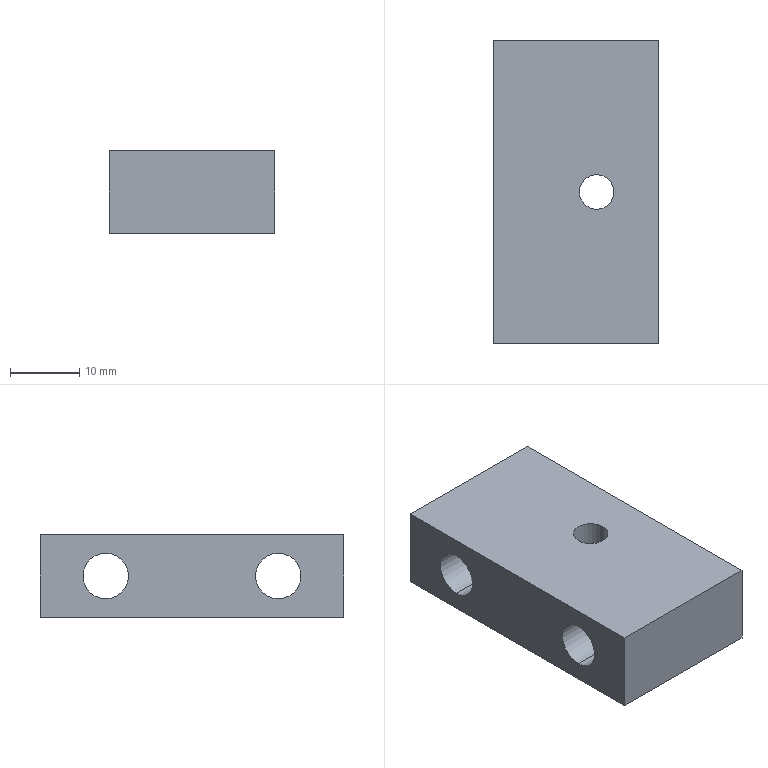Part | STEP file | 1 solid | 18 faces | box 24 x 44 x 12 mm | volume 10016 mm3 | cylinder 10 | plane 8 | commonest cylinder face diameters 6.6 x4 11 x4 5 x2
STEP:
#1=CARTESIAN_POINT('',(0.,0.,0.));
#2=DIRECTION('',(0.,0.,1.));
#3=DIRECTION('',(1.,0.,0.));
#4=AXIS2_PLACEMENT_3D('',#1,#2,#3);
#5=CARTESIAN_POINT('',(17.5,0.,-6.));
#6=VERTEX_POINT('',#5);
#7=CARTESIAN_POINT('',(17.5,0.,6.));
#8=VERTEX_POINT('',#7);
#9=CARTESIAN_POINT('',(17.5,0.,6.));
#10=DIRECTION('',(0.,0.,1.));
#11=VECTOR('',#10,1.);
#12=LINE('',#9,#11);
#13=CARTESIAN_POINT('',(15.,0.,6.));
#14=DIRECTION('',(0.,0.,1.));
#15=DIRECTION('',(1.,0.,0.));
#16=AXIS2_PLACEMENT_3D('',#13,#14,#15);
#17=CYLINDRICAL_SURFACE('',#16,2.5);
#18=CARTESIAN_POINT('',(6.283,0.));
#19=DIRECTION('',(0.,1.));
#20=VECTOR('',#19,1.);
#21=LINE('',#18,#20);
#22=(GEOMETRIC_REPRESENTATION_CONTEXT(2)PARAMETRIC_REPRESENTATION_CONTEXT()REPRESENTATION_CONTEXT('',''));
#23=DEFINITIONAL_REPRESENTATION('',(#21),#22);
#24=PCURVE('',#17,#23);
#25=CARTESIAN_POINT('',(15.,0.,6.));
#26=DIRECTION('',(0.,0.,1.));
#27=DIRECTION('',(1.,0.,0.));
#28=AXIS2_PLACEMENT_3D('',#25,#26,#27);
#29=CYLINDRICAL_SURFACE('',#28,2.5);
#30=CARTESIAN_POINT('',(0.,0.));
#31=DIRECTION('',(0.,1.));
#32=VECTOR('',#31,1.);
#33=LINE('',#30,#32);
#34=(GEOMETRIC_REPRESENTATION_CONTEXT(2)PARAMETRIC_REPRESENTATION_CONTEXT()REPRESENTATION_CONTEXT('',''));
#35=DEFINITIONAL_REPRESENTATION('',(#33),#34);
#36=PCURVE('',#29,#35);
#37=SURFACE_CURVE('',#12,(#24,#36),.PCURVE_S1.);
#38=EDGE_CURVE('',#6,#8,#37,.T.);
#39=ORIENTED_EDGE('',*,*,#38,.T.);
#40=CARTESIAN_POINT('',(12.5,0.,6.));
#41=VERTEX_POINT('',#40);
#42=CARTESIAN_POINT('',(15.,0.,6.));
#43=DIRECTION('',(0.,0.,1.));
#44=DIRECTION('',(1.,0.,0.));
#45=AXIS2_PLACEMENT_3D('',#42,#43,#44);
#46=CIRCLE('',#45,2.5);
#47=CARTESIAN_POINT('',(0.,0.));
#48=DIRECTION('',(1.,0.));
#49=VECTOR('',#48,1.);
#50=LINE('',#47,#49);
#51=(GEOMETRIC_REPRESENTATION_CONTEXT(2)PARAMETRIC_REPRESENTATION_CONTEXT()REPRESENTATION_CONTEXT('',''));
#52=DEFINITIONAL_REPRESENTATION('',(#50),#51);
#53=PCURVE('',#17,#52);
#54=CARTESIAN_POINT('',(24.,-22.,6.));
#55=DIRECTION('',(0.,0.,-1.));
#56=DIRECTION('',(-1.,0.,0.));
#57=AXIS2_PLACEMENT_3D('',#54,#55,#56);
#58=PLANE('',#57);
#59=CARTESIAN_POINT('',(6.5,22.));
#60=CARTESIAN_POINT('',(6.5,26.33));
#61=CARTESIAN_POINT('',(10.25,24.165));
#62=CARTESIAN_POINT('',(14.,22.));
#63=CARTESIAN_POINT('',(10.25,19.835));
#64=CARTESIAN_POINT('',(6.5,17.67));
#65=CARTESIAN_POINT('',(6.5,22.));
#66=(BOUNDED_CURVE()B_SPLINE_CURVE(2,(#59,#60,#61,#62,#63,#64,#65),.UNSPECIFIED.,.T.,.F.)B_SPLINE_CURVE_WITH_KNOTS((1,2,2,2,2,1),(-2.094,0.,2.094,4.189,6.283,8.378),.UNSPECIFIED.)CURVE()GEOMETRIC_REPRESENTATION_ITEM()RATIONAL_B_SPLINE_CURVE((1.,0.5,1.,0.5,1.,0.5,1.))REPRESENTATION_ITEM(''));
#67=(GEOMETRIC_REPRESENTATION_CONTEXT(2)PARAMETRIC_REPRESENTATION_CONTEXT()REPRESENTATION_CONTEXT('',''));
#68=DEFINITIONAL_REPRESENTATION('',(#66),#67);
#69=PCURVE('',#58,#68);
#70=SURFACE_CURVE('',#46,(#53,#69),.PCURVE_S1.);
#71=EDGE_CURVE('',#41,#8,#70,.T.);
#72=ORIENTED_EDGE('',*,*,#71,.F.);
#73=CARTESIAN_POINT('',(12.5,0.,-6.));
#74=VERTEX_POINT('',#73);
#75=CARTESIAN_POINT('',(12.5,0.,6.));
#76=DIRECTION('',(0.,0.,1.));
#77=VECTOR('',#76,1.);
#78=LINE('',#75,#77);
#79=CARTESIAN_POINT('',(3.142,0.));
#80=DIRECTION('',(0.,1.));
#81=VECTOR('',#80,1.);
#82=LINE('',#79,#81);
#83=(GEOMETRIC_REPRESENTATION_CONTEXT(2)PARAMETRIC_REPRESENTATION_CONTEXT()REPRESENTATION_CONTEXT('',''));
#84=DEFINITIONAL_REPRESENTATION('',(#82),#83);
#85=PCURVE('',#17,#84);
#86=CARTESIAN_POINT('',(3.142,0.));
#87=DIRECTION('',(0.,1.));
#88=VECTOR('',#87,1.);
#89=LINE('',#86,#88);
#90=(GEOMETRIC_REPRESENTATION_CONTEXT(2)PARAMETRIC_REPRESENTATION_CONTEXT()REPRESENTATION_CONTEXT('',''));
#91=DEFINITIONAL_REPRESENTATION('',(#89),#90);
#92=PCURVE('',#29,#91);
#93=SURFACE_CURVE('',#78,(#85,#92),.PCURVE_S1.);
#94=EDGE_CURVE('',#74,#41,#93,.T.);
#95=ORIENTED_EDGE('',*,*,#94,.F.);
#96=CARTESIAN_POINT('',(15.,0.,-6.));
#97=DIRECTION('',(0.,0.,1.));
#98=DIRECTION('',(1.,0.,0.));
#99=AXIS2_PLACEMENT_3D('',#96,#97,#98);
#100=CIRCLE('',#99,2.5);
#101=CARTESIAN_POINT('',(0.,-12.));
#102=DIRECTION('',(1.,0.));
#103=VECTOR('',#102,1.);
#104=LINE('',#101,#103);
#105=(GEOMETRIC_REPRESENTATION_CONTEXT(2)PARAMETRIC_REPRESENTATION_CONTEXT()REPRESENTATION_CONTEXT('',''));
#106=DEFINITIONAL_REPRESENTATION('',(#104),#105);
#107=PCURVE('',#17,#106);
#108=CARTESIAN_POINT('',(24.,-22.,-6.));
#109=DIRECTION('',(0.,0.,1.));
#110=DIRECTION('',(1.,0.,0.));
#111=AXIS2_PLACEMENT_3D('',#108,#109,#110);
#112=PLANE('',#111);
#113=CARTESIAN_POINT('',(-9.,22.));
#114=DIRECTION('',(1.,0.));
#115=AXIS2_PLACEMENT_2D('',#113,#114);
#116=CIRCLE('',#115,2.5);
#117=(GEOMETRIC_REPRESENTATION_CONTEXT(2)PARAMETRIC_REPRESENTATION_CONTEXT()REPRESENTATION_CONTEXT('',''));
#118=DEFINITIONAL_REPRESENTATION('',(#116),#117);
#119=PCURVE('',#112,#118);
#120=SURFACE_CURVE('',#100,(#107,#119),.PCURVE_S1.);
#121=EDGE_CURVE('',#74,#6,#120,.T.);
#122=ORIENTED_EDGE('',*,*,#121,.T.);
#123=EDGE_LOOP('',(#39,#72,#95,#122));
#124=FACE_BOUND('',#123,.F.);
#125=ADVANCED_FACE('',(#124),#17,.F.);
#126=CARTESIAN_POINT('',(17.6,12.5,-5.5));
#127=VERTEX_POINT('',#126);
#128=CARTESIAN_POINT('',(24.,12.5,-5.5));
#129=VERTEX_POINT('',#128);
#130=CARTESIAN_POINT('',(24.,12.5,-5.5));
#131=DIRECTION('',(1.,0.,0.));
#132=VECTOR('',#131,1.);
#133=LINE('',#130,#132);
#134=CARTESIAN_POINT('',(24.,12.5,0.));
#135=DIRECTION('',(1.,0.,0.));
#136=DIRECTION('',(0.,0.,-1.));
#137=AXIS2_PLACEMENT_3D('',#134,#135,#136);
#138=CYLINDRICAL_SURFACE('',#137,5.5);
#139=CARTESIAN_POINT('',(6.283,0.));
#140=DIRECTION('',(0.,1.));
#141=VECTOR('',#140,1.);
#142=LINE('',#139,#141);
#143=(GEOMETRIC_REPRESENTATION_CONTEXT(2)PARAMETRIC_REPRESENTATION_CONTEXT()REPRESENTATION_CONTEXT('',''));
#144=DEFINITIONAL_REPRESENTATION('',(#142),#143);
#145=PCURVE('',#138,#144);
#146=CARTESIAN_POINT('',(24.,12.5,0.));
#147=DIRECTION('',(1.,0.,0.));
#148=DIRECTION('',(0.,0.,-1.));
#149=AXIS2_PLACEMENT_3D('',#146,#147,#148);
#150=CYLINDRICAL_SURFACE('',#149,5.5);
#151=CARTESIAN_POINT('',(0.,0.));
#152=DIRECTION('',(0.,1.));
#153=VECTOR('',#152,1.);
#154=LINE('',#151,#153);
#155=(GEOMETRIC_REPRESENTATION_CONTEXT(2)PARAMETRIC_REPRESENTATION_CONTEXT()REPRESENTATION_CONTEXT('',''));
#156=DEFINITIONAL_REPRESENTATION('',(#154),#155);
#157=PCURVE('',#150,#156);
#158=SURFACE_CURVE('',#133,(#145,#157),.PCURVE_S1.);
#159=EDGE_CURVE('',#127,#129,#158,.T.);
#160=ORIENTED_EDGE('',*,*,#159,.T.);
#161=CARTESIAN_POINT('',(24.,12.5,5.5));
#162=VERTEX_POINT('',#161);
#163=CARTESIAN_POINT('',(24.,12.5,0.));
#164=DIRECTION('',(1.,0.,0.));
#165=DIRECTION('',(0.,0.,-1.));
#166=AXIS2_PLACEMENT_3D('',#163,#164,#165);
#167=CIRCLE('',#166,5.5);
#168=CARTESIAN_POINT('',(0.,0.));
#169=DIRECTION('',(1.,0.));
#170=VECTOR('',#169,1.);
#171=LINE('',#168,#170);
#172=(GEOMETRIC_REPRESENTATION_CONTEXT(2)PARAMETRIC_REPRESENTATION_CONTEXT()REPRESENTATION_CONTEXT('',''));
#173=DEFINITIONAL_REPRESENTATION('',(#171),#172);
#174=PCURVE('',#138,#173);
#175=CARTESIAN_POINT('',(24.,0.,0.));
#176=DIRECTION('',(1.,0.,0.));
#177=DIRECTION('',(0.,0.,-1.));
#178=AXIS2_PLACEMENT_3D('',#175,#176,#177);
#179=PLANE('',#178);
#180=CARTESIAN_POINT('',(0.,12.5));
#181=DIRECTION('',(1.,0.));
#182=AXIS2_PLACEMENT_2D('',#180,#181);
#183=CIRCLE('',#182,5.5);
#184=(GEOMETRIC_REPRESENTATION_CONTEXT(2)PARAMETRIC_REPRESENTATION_CONTEXT()REPRESENTATION_CONTEXT('',''));
#185=DEFINITIONAL_REPRESENTATION('',(#183),#184);
#186=PCURVE('',#179,#185);
#187=SURFACE_CURVE('',#167,(#174,#186),.PCURVE_S1.);
#188=EDGE_CURVE('',#162,#129,#187,.T.);
#189=ORIENTED_EDGE('',*,*,#188,.F.);
#190=CARTESIAN_POINT('',(17.6,12.5,5.5));
#191=VERTEX_POINT('',#190);
#192=CARTESIAN_POINT('',(24.,12.5,5.5));
#193=DIRECTION('',(1.,0.,0.));
#194=VECTOR('',#193,1.);
#195=LINE('',#192,#194);
#196=CARTESIAN_POINT('',(3.142,0.));
#197=DIRECTION('',(0.,1.));
#198=VECTOR('',#197,1.);
#199=LINE('',#196,#198);
#200=(GEOMETRIC_REPRESENTATION_CONTEXT(2)PARAMETRIC_REPRESENTATION_CONTEXT()REPRESENTATION_CONTEXT('',''));
#201=DEFINITIONAL_REPRESENTATION('',(#199),#200);
#202=PCURVE('',#138,#201);
#203=CARTESIAN_POINT('',(3.142,0.));
#204=DIRECTION('',(0.,1.));
#205=VECTOR('',#204,1.);
#206=LINE('',#203,#205);
#207=(GEOMETRIC_REPRESENTATION_CONTEXT(2)PARAMETRIC_REPRESENTATION_CONTEXT()REPRESENTATION_CONTEXT('',''));
#208=DEFINITIONAL_REPRESENTATION('',(#206),#207);
#209=PCURVE('',#150,#208);
#210=SURFACE_CURVE('',#195,(#202,#209),.PCURVE_S1.);
#211=EDGE_CURVE('',#191,#162,#210,.T.);
#212=ORIENTED_EDGE('',*,*,#211,.F.);
#213=CARTESIAN_POINT('',(17.6,12.5,0.));
#214=DIRECTION('',(1.,0.,0.));
#215=DIRECTION('',(0.,0.,-1.));
#216=AXIS2_PLACEMENT_3D('',#213,#214,#215);
#217=CIRCLE('',#216,5.5);
#218=CARTESIAN_POINT('',(0.,-6.4));
#219=DIRECTION('',(1.,0.));
#220=VECTOR('',#219,1.);
#221=LINE('',#218,#220);
#222=(GEOMETRIC_REPRESENTATION_CONTEXT(2)PARAMETRIC_REPRESENTATION_CONTEXT()REPRESENTATION_CONTEXT('',''));
#223=DEFINITIONAL_REPRESENTATION('',(#221),#222);
#224=PCURVE('',#138,#223);
#225=CARTESIAN_POINT('',(17.6,15.8,0.));
#226=DIRECTION('',(-1.,0.,0.));
#227=DIRECTION('',(0.,0.,1.));
#228=AXIS2_PLACEMENT_3D('',#225,#226,#227);
#229=PLANE('',#228);
#230=CARTESIAN_POINT('',(-5.5,-3.3));
#231=CARTESIAN_POINT('',(-5.5,6.226));
#232=CARTESIAN_POINT('',(2.75,1.463));
#233=CARTESIAN_POINT('',(11.,-3.3));
#234=CARTESIAN_POINT('',(2.75,-8.063));
#235=CARTESIAN_POINT('',(-5.5,-12.826));
#236=CARTESIAN_POINT('',(-5.5,-3.3));
#237=(BOUNDED_CURVE()B_SPLINE_CURVE(2,(#230,#231,#232,#233,#234,#235,#236),.UNSPECIFIED.,.T.,.F.)B_SPLINE_CURVE_WITH_KNOTS((1,2,2,2,2,1),(-2.094,0.,2.094,4.189,6.283,8.378),.UNSPECIFIED.)CURVE()GEOMETRIC_REPRESENTATION_ITEM()RATIONAL_B_SPLINE_CURVE((1.,0.5,1.,0.5,1.,0.5,1.))REPRESENTATION_ITEM(''));
#238=(GEOMETRIC_REPRESENTATION_CONTEXT(2)PARAMETRIC_REPRESENTATION_CONTEXT()REPRESENTATION_CONTEXT('',''));
#239=DEFINITIONAL_REPRESENTATION('',(#237),#238);
#240=PCURVE('',#229,#239);
#241=SURFACE_CURVE('',#217,(#224,#240),.PCURVE_S1.);
#242=EDGE_CURVE('',#191,#127,#241,.T.);
#243=ORIENTED_EDGE('',*,*,#242,.T.);
#244=EDGE_LOOP('',(#160,#189,#212,#243));
#245=FACE_BOUND('',#244,.F.);
#246=ADVANCED_FACE('',(#245),#138,.F.);
#247=CARTESIAN_POINT('',(0.,12.5,-3.3));
#248=VERTEX_POINT('',#247);
#249=CARTESIAN_POINT('',(17.6,12.5,-3.3));
#250=VERTEX_POINT('',#249);
#251=CARTESIAN_POINT('',(24.,12.5,-3.3));
#252=DIRECTION('',(1.,0.,0.));
#253=VECTOR('',#252,1.);
#254=LINE('',#251,#253);
#255=CARTESIAN_POINT('',(24.,12.5,0.));
#256=DIRECTION('',(1.,0.,0.));
#257=DIRECTION('',(0.,0.,-1.));
#258=AXIS2_PLACEMENT_3D('',#255,#256,#257);
#259=CYLINDRICAL_SURFACE('',#258,3.3);
#260=CARTESIAN_POINT('',(6.283,0.));
#261=DIRECTION('',(0.,1.));
#262=VECTOR('',#261,1.);
#263=LINE('',#260,#262);
#264=(GEOMETRIC_REPRESENTATION_CONTEXT(2)PARAMETRIC_REPRESENTATION_CONTEXT()REPRESENTATION_CONTEXT('',''));
#265=DEFINITIONAL_REPRESENTATION('',(#263),#264);
#266=PCURVE('',#259,#265);
#267=CARTESIAN_POINT('',(24.,12.5,0.));
#268=DIRECTION('',(1.,0.,0.));
#269=DIRECTION('',(0.,0.,-1.));
#270=AXIS2_PLACEMENT_3D('',#267,#268,#269);
#271=CYLINDRICAL_SURFACE('',#270,3.3);
#272=CARTESIAN_POINT('',(0.,0.));
#273=DIRECTION('',(0.,1.));
#274=VECTOR('',#273,1.);
#275=LINE('',#272,#274);
#276=(GEOMETRIC_REPRESENTATION_CONTEXT(2)PARAMETRIC_REPRESENTATION_CONTEXT()REPRESENTATION_CONTEXT('',''));
#277=DEFINITIONAL_REPRESENTATION('',(#275),#276);
#278=PCURVE('',#271,#277);
#279=SURFACE_CURVE('',#254,(#266,#278),.PCURVE_S1.);
#280=EDGE_CURVE('',#248,#250,#279,.T.);
#281=ORIENTED_EDGE('',*,*,#280,.T.);
#282=CARTESIAN_POINT('',(17.6,12.5,3.3));
#283=VERTEX_POINT('',#282);
#284=CARTESIAN_POINT('',(17.6,12.5,0.));
#285=DIRECTION('',(1.,0.,0.));
#286=DIRECTION('',(0.,0.,-1.));
#287=AXIS2_PLACEMENT_3D('',#284,#285,#286);
#288=CIRCLE('',#287,3.3);
#289=CARTESIAN_POINT('',(0.,-6.4));
#290=DIRECTION('',(1.,0.));
#291=VECTOR('',#290,1.);
#292=LINE('',#289,#291);
#293=(GEOMETRIC_REPRESENTATION_CONTEXT(2)PARAMETRIC_REPRESENTATION_CONTEXT()REPRESENTATION_CONTEXT('',''));
#294=DEFINITIONAL_REPRESENTATION('',(#292),#293);
#295=PCURVE('',#259,#294);
#296=CARTESIAN_POINT('',(-3.3,-3.3));
#297=CARTESIAN_POINT('',(-3.3,2.416));
#298=CARTESIAN_POINT('',(1.65,-0.4421));
#299=CARTESIAN_POINT('',(6.6,-3.3));
#300=CARTESIAN_POINT('',(1.65,-6.158));
#301=CARTESIAN_POINT('',(-3.3,-9.016));
#302=CARTESIAN_POINT('',(-3.3,-3.3));
#303=(BOUNDED_CURVE()B_SPLINE_CURVE(2,(#296,#297,#298,#299,#300,#301,#302),.UNSPECIFIED.,.T.,.F.)B_SPLINE_CURVE_WITH_KNOTS((1,2,2,2,2,1),(-2.094,0.,2.094,4.189,6.283,8.378),.UNSPECIFIED.)CURVE()GEOMETRIC_REPRESENTATION_ITEM()RATIONAL_B_SPLINE_CURVE((1.,0.5,1.,0.5,1.,0.5,1.))REPRESENTATION_ITEM(''));
#304=(GEOMETRIC_REPRESENTATION_CONTEXT(2)PARAMETRIC_REPRESENTATION_CONTEXT()REPRESENTATION_CONTEXT('',''));
#305=DEFINITIONAL_REPRESENTATION('',(#303),#304);
#306=PCURVE('',#229,#305);
#307=SURFACE_CURVE('',#288,(#295,#306),.PCURVE_S1.);
#308=EDGE_CURVE('',#283,#250,#307,.T.);
#309=ORIENTED_EDGE('',*,*,#308,.F.);
#310=CARTESIAN_POINT('',(0.,12.5,3.3));
#311=VERTEX_POINT('',#310);
#312=CARTESIAN_POINT('',(24.,12.5,3.3));
#313=DIRECTION('',(1.,0.,0.));
#314=VECTOR('',#313,1.);
#315=LINE('',#312,#314);
#316=CARTESIAN_POINT('',(3.142,0.));
#317=DIRECTION('',(0.,1.));
#318=VECTOR('',#317,1.);
#319=LINE('',#316,#318);
#320=(GEOMETRIC_REPRESENTATION_CONTEXT(2)PARAMETRIC_REPRESENTATION_CONTEXT()REPRESENTATION_CONTEXT('',''));
#321=DEFINITIONAL_REPRESENTATION('',(#319),#320);
#322=PCURVE('',#259,#321);
#323=CARTESIAN_POINT('',(3.142,0.));
#324=DIRECTION('',(0.,1.));
#325=VECTOR('',#324,1.);
#326=LINE('',#323,#325);
#327=(GEOMETRIC_REPRESENTATION_CONTEXT(2)PARAMETRIC_REPRESENTATION_CONTEXT()REPRESENTATION_CONTEXT('',''));
#328=DEFINITIONAL_REPRESENTATION('',(#326),#327);
#329=PCURVE('',#271,#328);
#330=SURFACE_CURVE('',#315,(#322,#329),.PCURVE_S1.);
#331=EDGE_CURVE('',#311,#283,#330,.T.);
#332=ORIENTED_EDGE('',*,*,#331,.F.);
#333=CARTESIAN_POINT('',(0.,12.5,0.));
#334=DIRECTION('',(1.,0.,0.));
#335=DIRECTION('',(0.,0.,-1.));
#336=AXIS2_PLACEMENT_3D('',#333,#334,#335);
#337=CIRCLE('',#336,3.3);
#338=CARTESIAN_POINT('',(0.,-24.));
#339=DIRECTION('',(1.,0.));
#340=VECTOR('',#339,1.);
#341=LINE('',#338,#340);
#342=(GEOMETRIC_REPRESENTATION_CONTEXT(2)PARAMETRIC_REPRESENTATION_CONTEXT()REPRESENTATION_CONTEXT('',''));
#343=DEFINITIONAL_REPRESENTATION('',(#341),#342);
#344=PCURVE('',#259,#343);
#345=CARTESIAN_POINT('',(0.,0.,0.));
#346=DIRECTION('',(1.,0.,0.));
#347=DIRECTION('',(0.,0.,-1.));
#348=AXIS2_PLACEMENT_3D('',#345,#346,#347);
#349=PLANE('',#348);
#350=CARTESIAN_POINT('',(0.,12.5));
#351=DIRECTION('',(1.,0.));
#352=AXIS2_PLACEMENT_2D('',#350,#351);
#353=CIRCLE('',#352,3.3);
#354=(GEOMETRIC_REPRESENTATION_CONTEXT(2)PARAMETRIC_REPRESENTATION_CONTEXT()REPRESENTATION_CONTEXT('',''));
#355=DEFINITIONAL_REPRESENTATION('',(#353),#354);
#356=PCURVE('',#349,#355);
#357=SURFACE_CURVE('',#337,(#344,#356),.PCURVE_S1.);
#358=EDGE_CURVE('',#311,#248,#357,.T.);
#359=ORIENTED_EDGE('',*,*,#358,.T.);
#360=EDGE_LOOP('',(#281,#309,#332,#359));
#361=FACE_BOUND('',#360,.F.);
#362=ADVANCED_FACE('',(#361),#259,.F.);
#363=CARTESIAN_POINT('',(17.6,-12.5,-5.5));
#364=VERTEX_POINT('',#363);
#365=CARTESIAN_POINT('',(24.,-12.5,-5.5));
#366=VERTEX_POINT('',#365);
#367=CARTESIAN_POINT('',(24.,-12.5,-5.5));
#368=DIRECTION('',(1.,0.,0.));
#369=VECTOR('',#368,1.);
#370=LINE('',#367,#369);
#371=CARTESIAN_POINT('',(24.,-12.5,0.));
#372=DIRECTION('',(1.,0.,0.));
#373=DIRECTION('',(0.,0.,-1.));
#374=AXIS2_PLACEMENT_3D('',#371,#372,#373);
#375=CYLINDRICAL_SURFACE('',#374,5.5);
#376=CARTESIAN_POINT('',(6.283,0.));
#377=DIRECTION('',(0.,1.));
#378=VECTOR('',#377,1.);
#379=LINE('',#376,#378);
#380=(GEOMETRIC_REPRESENTATION_CONTEXT(2)PARAMETRIC_REPRESENTATION_CONTEXT()REPRESENTATION_CONTEXT('',''));
#381=DEFINITIONAL_REPRESENTATION('',(#379),#380);
#382=PCURVE('',#375,#381);
#383=CARTESIAN_POINT('',(24.,-12.5,0.));
#384=DIRECTION('',(1.,0.,0.));
#385=DIRECTION('',(0.,0.,-1.));
#386=AXIS2_PLACEMENT_3D('',#383,#384,#385);
#387=CYLINDRICAL_SURFACE('',#386,5.5);
#388=CARTESIAN_POINT('',(0.,0.));
#389=DIRECTION('',(0.,1.));
#390=VECTOR('',#389,1.);
#391=LINE('',#388,#390);
#392=(GEOMETRIC_REPRESENTATION_CONTEXT(2)PARAMETRIC_REPRESENTATION_CONTEXT()REPRESENTATION_CONTEXT('',''));
#393=DEFINITIONAL_REPRESENTATION('',(#391),#392);
#394=PCURVE('',#387,#393);
#395=SURFACE_CURVE('',#370,(#382,#394),.PCURVE_S1.);
#396=EDGE_CURVE('',#364,#366,#395,.T.);
#397=ORIENTED_EDGE('',*,*,#396,.T.);
#398=CARTESIAN_POINT('',(24.,-12.5,5.5));
#399=VERTEX_POINT('',#398);
#400=CARTESIAN_POINT('',(24.,-12.5,0.));
#401=DIRECTION('',(1.,0.,0.));
#402=DIRECTION('',(0.,0.,-1.));
#403=AXIS2_PLACEMENT_3D('',#400,#401,#402);
#404=CIRCLE('',#403,5.5);
#405=CARTESIAN_POINT('',(0.,0.));
#406=DIRECTION('',(1.,0.));
#407=VECTOR('',#406,1.);
#408=LINE('',#405,#407);
#409=(GEOMETRIC_REPRESENTATION_CONTEXT(2)PARAMETRIC_REPRESENTATION_CONTEXT()REPRESENTATION_CONTEXT('',''));
#410=DEFINITIONAL_REPRESENTATION('',(#408),#409);
#411=PCURVE('',#375,#410);
#412=CARTESIAN_POINT('',(0.,-12.5));
#413=DIRECTION('',(1.,0.));
#414=AXIS2_PLACEMENT_2D('',#412,#413);
#415=CIRCLE('',#414,5.5);
#416=(GEOMETRIC_REPRESENTATION_CONTEXT(2)PARAMETRIC_REPRESENTATION_CONTEXT()REPRESENTATION_CONTEXT('',''));
#417=DEFINITIONAL_REPRESENTATION('',(#415),#416);
#418=PCURVE('',#179,#417);
#419=SURFACE_CURVE('',#404,(#411,#418),.PCURVE_S1.);
#420=EDGE_CURVE('',#399,#366,#419,.T.);
#421=ORIENTED_EDGE('',*,*,#420,.F.);
#422=CARTESIAN_POINT('',(17.6,-12.5,5.5));
#423=VERTEX_POINT('',#422);
#424=CARTESIAN_POINT('',(24.,-12.5,5.5));
#425=DIRECTION('',(1.,0.,0.));
#426=VECTOR('',#425,1.);
#427=LINE('',#424,#426);
#428=CARTESIAN_POINT('',(3.142,0.));
#429=DIRECTION('',(0.,1.));
#430=VECTOR('',#429,1.);
#431=LINE('',#428,#430);
#432=(GEOMETRIC_REPRESENTATION_CONTEXT(2)PARAMETRIC_REPRESENTATION_CONTEXT()REPRESENTATION_CONTEXT('',''));
#433=DEFINITIONAL_REPRESENTATION('',(#431),#432);
#434=PCURVE('',#375,#433);
#435=CARTESIAN_POINT('',(3.142,0.));
#436=DIRECTION('',(0.,1.));
#437=VECTOR('',#436,1.);
#438=LINE('',#435,#437);
#439=(GEOMETRIC_REPRESENTATION_CONTEXT(2)PARAMETRIC_REPRESENTATION_CONTEXT()REPRESENTATION_CONTEXT('',''));
#440=DEFINITIONAL_REPRESENTATION('',(#438),#439);
#441=PCURVE('',#387,#440);
#442=SURFACE_CURVE('',#427,(#434,#441),.PCURVE_S1.);
#443=EDGE_CURVE('',#423,#399,#442,.T.);
#444=ORIENTED_EDGE('',*,*,#443,.F.);
#445=CARTESIAN_POINT('',(17.6,-12.5,0.));
#446=DIRECTION('',(1.,0.,0.));
#447=DIRECTION('',(0.,0.,-1.));
#448=AXIS2_PLACEMENT_3D('',#445,#446,#447);
#449=CIRCLE('',#448,5.5);
#450=CARTESIAN_POINT('',(0.,-6.4));
#451=DIRECTION('',(1.,0.));
#452=VECTOR('',#451,1.);
#453=LINE('',#450,#452);
#454=(GEOMETRIC_REPRESENTATION_CONTEXT(2)PARAMETRIC_REPRESENTATION_CONTEXT()REPRESENTATION_CONTEXT('',''));
#455=DEFINITIONAL_REPRESENTATION('',(#453),#454);
#456=PCURVE('',#375,#455);
#457=CARTESIAN_POINT('',(17.6,-9.2,0.));
#458=DIRECTION('',(-1.,0.,0.));
#459=DIRECTION('',(0.,0.,1.));
#460=AXIS2_PLACEMENT_3D('',#457,#458,#459);
#461=PLANE('',#460);
#462=CARTESIAN_POINT('',(-5.5,-3.3));
#463=CARTESIAN_POINT('',(-5.5,6.226));
#464=CARTESIAN_POINT('',(2.75,1.463));
#465=CARTESIAN_POINT('',(11.,-3.3));
#466=CARTESIAN_POINT('',(2.75,-8.063));
#467=CARTESIAN_POINT('',(-5.5,-12.826));
#468=CARTESIAN_POINT('',(-5.5,-3.3));
#469=(BOUNDED_CURVE()B_SPLINE_CURVE(2,(#462,#463,#464,#465,#466,#467,#468),.UNSPECIFIED.,.T.,.F.)B_SPLINE_CURVE_WITH_KNOTS((1,2,2,2,2,1),(-2.094,0.,2.094,4.189,6.283,8.378),.UNSPECIFIED.)CURVE()GEOMETRIC_REPRESENTATION_ITEM()RATIONAL_B_SPLINE_CURVE((1.,0.5,1.,0.5,1.,0.5,1.))REPRESENTATION_ITEM(''));
#470=(GEOMETRIC_REPRESENTATION_CONTEXT(2)PARAMETRIC_REPRESENTATION_CONTEXT()REPRESENTATION_CONTEXT('',''));
#471=DEFINITIONAL_REPRESENTATION('',(#469),#470);
#472=PCURVE('',#461,#471);
#473=SURFACE_CURVE('',#449,(#456,#472),.PCURVE_S1.);
#474=EDGE_CURVE('',#423,#364,#473,.T.);
#475=ORIENTED_EDGE('',*,*,#474,.T.);
#476=EDGE_LOOP('',(#397,#421,#444,#475));
#477=FACE_BOUND('',#476,.F.);
#478=ADVANCED_FACE('',(#477),#375,.F.);
#479=CARTESIAN_POINT('',(0.,-12.5,-3.3));
#480=VERTEX_POINT('',#479);
#481=CARTESIAN_POINT('',(17.6,-12.5,-3.3));
#482=VERTEX_POINT('',#481);
#483=CARTESIAN_POINT('',(24.,-12.5,-3.3));
#484=DIRECTION('',(1.,0.,0.));
#485=VECTOR('',#484,1.);
#486=LINE('',#483,#485);
#487=CARTESIAN_POINT('',(24.,-12.5,0.));
#488=DIRECTION('',(1.,0.,0.));
#489=DIRECTION('',(0.,0.,-1.));
#490=AXIS2_PLACEMENT_3D('',#487,#488,#489);
#491=CYLINDRICAL_SURFACE('',#490,3.3);
#492=CARTESIAN_POINT('',(6.283,0.));
#493=DIRECTION('',(0.,1.));
#494=VECTOR('',#493,1.);
#495=LINE('',#492,#494);
#496=(GEOMETRIC_REPRESENTATION_CONTEXT(2)PARAMETRIC_REPRESENTATION_CONTEXT()REPRESENTATION_CONTEXT('',''));
#497=DEFINITIONAL_REPRESENTATION('',(#495),#496);
#498=PCURVE('',#491,#497);
#499=CARTESIAN_POINT('',(24.,-12.5,0.));
#500=DIRECTION('',(1.,0.,0.));
#501=DIRECTION('',(0.,0.,-1.));
#502=AXIS2_PLACEMENT_3D('',#499,#500,#501);
#503=CYLINDRICAL_SURFACE('',#502,3.3);
#504=CARTESIAN_POINT('',(0.,0.));
#505=DIRECTION('',(0.,1.));
#506=VECTOR('',#505,1.);
#507=LINE('',#504,#506);
#508=(GEOMETRIC_REPRESENTATION_CONTEXT(2)PARAMETRIC_REPRESENTATION_CONTEXT()REPRESENTATION_CONTEXT('',''));
#509=DEFINITIONAL_REPRESENTATION('',(#507),#508);
#510=PCURVE('',#503,#509);
#511=SURFACE_CURVE('',#486,(#498,#510),.PCURVE_S1.);
#512=EDGE_CURVE('',#480,#482,#511,.T.);
#513=ORIENTED_EDGE('',*,*,#512,.T.);
#514=CARTESIAN_POINT('',(17.6,-12.5,3.3));
#515=VERTEX_POINT('',#514);
#516=CARTESIAN_POINT('',(17.6,-12.5,0.));
#517=DIRECTION('',(1.,0.,0.));
#518=DIRECTION('',(0.,0.,-1.));
#519=AXIS2_PLACEMENT_3D('',#516,#517,#518);
#520=CIRCLE('',#519,3.3);
#521=CARTESIAN_POINT('',(0.,-6.4));
#522=DIRECTION('',(1.,0.));
#523=VECTOR('',#522,1.);
#524=LINE('',#521,#523);
#525=(GEOMETRIC_REPRESENTATION_CONTEXT(2)PARAMETRIC_REPRESENTATION_CONTEXT()REPRESENTATION_CONTEXT('',''));
#526=DEFINITIONAL_REPRESENTATION('',(#524),#525);
#527=PCURVE('',#491,#526);
#528=CARTESIAN_POINT('',(-3.3,-3.3));
#529=CARTESIAN_POINT('',(-3.3,2.416));
#530=CARTESIAN_POINT('',(1.65,-0.4421));
#531=CARTESIAN_POINT('',(6.6,-3.3));
#532=CARTESIAN_POINT('',(1.65,-6.158));
#533=CARTESIAN_POINT('',(-3.3,-9.016));
#534=CARTESIAN_POINT('',(-3.3,-3.3));
#535=(BOUNDED_CURVE()B_SPLINE_CURVE(2,(#528,#529,#530,#531,#532,#533,#534),.UNSPECIFIED.,.T.,.F.)B_SPLINE_CURVE_WITH_KNOTS((1,2,2,2,2,1),(-2.094,0.,2.094,4.189,6.283,8.378),.UNSPECIFIED.)CURVE()GEOMETRIC_REPRESENTATION_ITEM()RATIONAL_B_SPLINE_CURVE((1.,0.5,1.,0.5,1.,0.5,1.))REPRESENTATION_ITEM(''));
#536=(GEOMETRIC_REPRESENTATION_CONTEXT(2)PARAMETRIC_REPRESENTATION_CONTEXT()REPRESENTATION_CONTEXT('',''));
#537=DEFINITIONAL_REPRESENTATION('',(#535),#536);
#538=PCURVE('',#461,#537);
#539=SURFACE_CURVE('',#520,(#527,#538),.PCURVE_S1.);
#540=EDGE_CURVE('',#515,#482,#539,.T.);
#541=ORIENTED_EDGE('',*,*,#540,.F.);
#542=CARTESIAN_POINT('',(0.,-12.5,3.3));
#543=VERTEX_POINT('',#542);
#544=CARTESIAN_POINT('',(24.,-12.5,3.3));
#545=DIRECTION('',(1.,0.,0.));
#546=VECTOR('',#545,1.);
#547=LINE('',#544,#546);
#548=CARTESIAN_POINT('',(3.142,0.));
#549=DIRECTION('',(0.,1.));
#550=VECTOR('',#549,1.);
#551=LINE('',#548,#550);
#552=(GEOMETRIC_REPRESENTATION_CONTEXT(2)PARAMETRIC_REPRESENTATION_CONTEXT()REPRESENTATION_CONTEXT('',''));
#553=DEFINITIONAL_REPRESENTATION('',(#551),#552);
#554=PCURVE('',#491,#553);
#555=CARTESIAN_POINT('',(3.142,0.));
#556=DIRECTION('',(0.,1.));
#557=VECTOR('',#556,1.);
#558=LINE('',#555,#557);
#559=(GEOMETRIC_REPRESENTATION_CONTEXT(2)PARAMETRIC_REPRESENTATION_CONTEXT()REPRESENTATION_CONTEXT('',''));
#560=DEFINITIONAL_REPRESENTATION('',(#558),#559);
#561=PCURVE('',#503,#560);
#562=SURFACE_CURVE('',#547,(#554,#561),.PCURVE_S1.);
#563=EDGE_CURVE('',#543,#515,#562,.T.);
#564=ORIENTED_EDGE('',*,*,#563,.F.);
#565=CARTESIAN_POINT('',(0.,-12.5,0.));
#566=DIRECTION('',(1.,0.,0.));
#567=DIRECTION('',(0.,0.,-1.));
#568=AXIS2_PLACEMENT_3D('',#565,#566,#567);
#569=CIRCLE('',#568,3.3);
#570=CARTESIAN_POINT('',(0.,-24.));
#571=DIRECTION('',(1.,0.));
#572=VECTOR('',#571,1.);
#573=LINE('',#570,#572);
#574=(GEOMETRIC_REPRESENTATION_CONTEXT(2)PARAMETRIC_REPRESENTATION_CONTEXT()REPRESENTATION_CONTEXT('',''));
#575=DEFINITIONAL_REPRESENTATION('',(#573),#574);
#576=PCURVE('',#491,#575);
#577=CARTESIAN_POINT('',(0.,-12.5));
#578=DIRECTION('',(1.,0.));
#579=AXIS2_PLACEMENT_2D('',#577,#578);
#580=CIRCLE('',#579,3.3);
#581=(GEOMETRIC_REPRESENTATION_CONTEXT(2)PARAMETRIC_REPRESENTATION_CONTEXT()REPRESENTATION_CONTEXT('',''));
#582=DEFINITIONAL_REPRESENTATION('',(#580),#581);
#583=PCURVE('',#349,#582);
#584=SURFACE_CURVE('',#569,(#576,#583),.PCURVE_S1.);
#585=EDGE_CURVE('',#543,#480,#584,.T.);
#586=ORIENTED_EDGE('',*,*,#585,.T.);
#587=EDGE_LOOP('',(#513,#541,#564,#586));
#588=FACE_BOUND('',#587,.F.);
#589=ADVANCED_FACE('',(#588),#491,.F.);
#590=CARTESIAN_POINT('',(15.,0.,6.));
#591=DIRECTION('',(0.,0.,1.));
#592=DIRECTION('',(1.,0.,0.));
#593=AXIS2_PLACEMENT_3D('',#590,#591,#592);
#594=CIRCLE('',#593,2.5);
#595=CARTESIAN_POINT('',(6.5,22.));
#596=CARTESIAN_POINT('',(6.5,26.33));
#597=CARTESIAN_POINT('',(10.25,24.165));
#598=CARTESIAN_POINT('',(14.,22.));
#599=CARTESIAN_POINT('',(10.25,19.835));
#600=CARTESIAN_POINT('',(6.5,17.67));
#601=CARTESIAN_POINT('',(6.5,22.));
#602=(BOUNDED_CURVE()B_SPLINE_CURVE(2,(#595,#596,#597,#598,#599,#600,#601),.UNSPECIFIED.,.T.,.F.)B_SPLINE_CURVE_WITH_KNOTS((1,2,2,2,2,1),(-2.094,0.,2.094,4.189,6.283,8.378),.UNSPECIFIED.)CURVE()GEOMETRIC_REPRESENTATION_ITEM()RATIONAL_B_SPLINE_CURVE((1.,0.5,1.,0.5,1.,0.5,1.))REPRESENTATION_ITEM(''));
#603=(GEOMETRIC_REPRESENTATION_CONTEXT(2)PARAMETRIC_REPRESENTATION_CONTEXT()REPRESENTATION_CONTEXT('',''));
#604=DEFINITIONAL_REPRESENTATION('',(#602),#603);
#605=PCURVE('',#58,#604);
#606=CARTESIAN_POINT('',(0.,0.));
#607=DIRECTION('',(1.,0.));
#608=VECTOR('',#607,1.);
#609=LINE('',#606,#608);
#610=(GEOMETRIC_REPRESENTATION_CONTEXT(2)PARAMETRIC_REPRESENTATION_CONTEXT()REPRESENTATION_CONTEXT('',''));
#611=DEFINITIONAL_REPRESENTATION('',(#609),#610);
#612=PCURVE('',#29,#611);
#613=SURFACE_CURVE('',#594,(#605,#612),.PCURVE_S1.);
#614=EDGE_CURVE('',#8,#41,#613,.T.);
#615=ORIENTED_EDGE('',*,*,#614,.F.);
#616=ORIENTED_EDGE('',*,*,#71,.F.);
#617=EDGE_LOOP('',(#615,#616));
#618=FACE_BOUND('',#617,.T.);
#619=CARTESIAN_POINT('',(0.,22.,6.));
#620=VERTEX_POINT('',#619);
#621=CARTESIAN_POINT('',(0.,-22.,6.));
#622=VERTEX_POINT('',#621);
#623=CARTESIAN_POINT('',(0.,-22.,6.));
#624=DIRECTION('',(0.,-1.,0.));
#625=VECTOR('',#624,1.);
#626=LINE('',#623,#625);
#627=CARTESIAN_POINT('',(24.,0.));
#628=DIRECTION('',(0.,-1.));
#629=VECTOR('',#628,1.);
#630=LINE('',#627,#629);
#631=(GEOMETRIC_REPRESENTATION_CONTEXT(2)PARAMETRIC_REPRESENTATION_CONTEXT()REPRESENTATION_CONTEXT('',''));
#632=DEFINITIONAL_REPRESENTATION('',(#630),#631);
#633=PCURVE('',#58,#632);
#634=CARTESIAN_POINT('',(-6.,-22.));
#635=DIRECTION('',(0.,-1.));
#636=VECTOR('',#635,1.);
#637=LINE('',#634,#636);
#638=(GEOMETRIC_REPRESENTATION_CONTEXT(2)PARAMETRIC_REPRESENTATION_CONTEXT()REPRESENTATION_CONTEXT('',''));
#639=DEFINITIONAL_REPRESENTATION('',(#637),#638);
#640=PCURVE('',#349,#639);
#641=SURFACE_CURVE('',#626,(#633,#640),.PCURVE_S1.);
#642=EDGE_CURVE('',#620,#622,#641,.T.);
#643=ORIENTED_EDGE('',*,*,#642,.T.);
#644=CARTESIAN_POINT('',(24.,-22.,6.));
#645=VERTEX_POINT('',#644);
#646=CARTESIAN_POINT('',(24.,-22.,6.));
#647=DIRECTION('',(-1.,0.,0.));
#648=VECTOR('',#647,1.);
#649=LINE('',#646,#648);
#650=CARTESIAN_POINT('',(0.,0.));
#651=DIRECTION('',(1.,0.));
#652=VECTOR('',#651,1.);
#653=LINE('',#650,#652);
#654=(GEOMETRIC_REPRESENTATION_CONTEXT(2)PARAMETRIC_REPRESENTATION_CONTEXT()REPRESENTATION_CONTEXT('',''));
#655=DEFINITIONAL_REPRESENTATION('',(#653),#654);
#656=PCURVE('',#58,#655);
#657=CARTESIAN_POINT('',(24.,-22.,-6.));
#658=DIRECTION('',(0.,1.,0.));
#659=DIRECTION('',(0.,0.,1.));
#660=AXIS2_PLACEMENT_3D('',#657,#658,#659);
#661=PLANE('',#660);
#662=CARTESIAN_POINT('',(12.,0.));
#663=DIRECTION('',(0.,-1.));
#664=VECTOR('',#663,1.);
#665=LINE('',#662,#664);
#666=(GEOMETRIC_REPRESENTATION_CONTEXT(2)PARAMETRIC_REPRESENTATION_CONTEXT()REPRESENTATION_CONTEXT('',''));
#667=DEFINITIONAL_REPRESENTATION('',(#665),#666);
#668=PCURVE('',#661,#667);
#669=SURFACE_CURVE('',#649,(#656,#668),.PCURVE_S1.);
#670=EDGE_CURVE('',#645,#622,#669,.T.);
#671=ORIENTED_EDGE('',*,*,#670,.F.);
#672=CARTESIAN_POINT('',(24.,22.,6.));
#673=VERTEX_POINT('',#672);
#674=CARTESIAN_POINT('',(24.,-22.,6.));
#675=DIRECTION('',(0.,-1.,0.));
#676=VECTOR('',#675,1.);
#677=LINE('',#674,#676);
#678=CARTESIAN_POINT('',(0.,0.));
#679=DIRECTION('',(0.,-1.));
#680=VECTOR('',#679,1.);
#681=LINE('',#678,#680);
#682=(GEOMETRIC_REPRESENTATION_CONTEXT(2)PARAMETRIC_REPRESENTATION_CONTEXT()REPRESENTATION_CONTEXT('',''));
#683=DEFINITIONAL_REPRESENTATION('',(#681),#682);
#684=PCURVE('',#58,#683);
#685=CARTESIAN_POINT('',(-6.,-22.));
#686=DIRECTION('',(0.,-1.));
#687=VECTOR('',#686,1.);
#688=LINE('',#685,#687);
#689=(GEOMETRIC_REPRESENTATION_CONTEXT(2)PARAMETRIC_REPRESENTATION_CONTEXT()REPRESENTATION_CONTEXT('',''));
#690=DEFINITIONAL_REPRESENTATION('',(#688),#689);
#691=PCURVE('',#179,#690);
#692=SURFACE_CURVE('',#677,(#684,#691),.PCURVE_S1.);
#693=EDGE_CURVE('',#673,#645,#692,.T.);
#694=ORIENTED_EDGE('',*,*,#693,.F.);
#695=CARTESIAN_POINT('',(24.,22.,6.));
#696=DIRECTION('',(-1.,0.,0.));
#697=VECTOR('',#696,1.);
#698=LINE('',#695,#697);
#699=CARTESIAN_POINT('',(0.,44.));
#700=DIRECTION('',(1.,0.));
#701=VECTOR('',#700,1.);
#702=LINE('',#699,#701);
#703=(GEOMETRIC_REPRESENTATION_CONTEXT(2)PARAMETRIC_REPRESENTATION_CONTEXT()REPRESENTATION_CONTEXT('',''));
#704=DEFINITIONAL_REPRESENTATION('',(#702),#703);
#705=PCURVE('',#58,#704);
#706=CARTESIAN_POINT('',(24.,22.,-6.));
#707=DIRECTION('',(0.,-1.,0.));
#708=DIRECTION('',(0.,0.,-1.));
#709=AXIS2_PLACEMENT_3D('',#706,#707,#708);
#710=PLANE('',#709);
#711=CARTESIAN_POINT('',(-12.,0.));
#712=DIRECTION('',(0.,-1.));
#713=VECTOR('',#712,1.);
#714=LINE('',#711,#713);
#715=(GEOMETRIC_REPRESENTATION_CONTEXT(2)PARAMETRIC_REPRESENTATION_CONTEXT()REPRESENTATION_CONTEXT('',''));
#716=DEFINITIONAL_REPRESENTATION('',(#714),#715);
#717=PCURVE('',#710,#716);
#718=SURFACE_CURVE('',#698,(#705,#717),.PCURVE_S1.);
#719=EDGE_CURVE('',#673,#620,#718,.T.);
#720=ORIENTED_EDGE('',*,*,#719,.T.);
#721=EDGE_LOOP('',(#643,#671,#694,#720));
#722=FACE_BOUND('',#721,.T.);
#723=ADVANCED_FACE('',(#618,#722),#58,.F.);
#724=CARTESIAN_POINT('',(0.,-22.,-6.));
#725=VERTEX_POINT('',#724);
#726=CARTESIAN_POINT('',(0.,-22.,-6.));
#727=DIRECTION('',(0.,0.,-1.));
#728=VECTOR('',#727,1.);
#729=LINE('',#726,#728);
#730=CARTESIAN_POINT('',(0.,-24.));
#731=DIRECTION('',(-1.,0.));
#732=VECTOR('',#731,1.);
#733=LINE('',#730,#732);
#734=(GEOMETRIC_REPRESENTATION_CONTEXT(2)PARAMETRIC_REPRESENTATION_CONTEXT()REPRESENTATION_CONTEXT('',''));
#735=DEFINITIONAL_REPRESENTATION('',(#733),#734);
#736=PCURVE('',#661,#735);
#737=CARTESIAN_POINT('',(6.,-22.));
#738=DIRECTION('',(1.,0.));
#739=VECTOR('',#738,1.);
#740=LINE('',#737,#739);
#741=(GEOMETRIC_REPRESENTATION_CONTEXT(2)PARAMETRIC_REPRESENTATION_CONTEXT()REPRESENTATION_CONTEXT('',''));
#742=DEFINITIONAL_REPRESENTATION('',(#740),#741);
#743=PCURVE('',#349,#742);
#744=SURFACE_CURVE('',#729,(#736,#743),.PCURVE_S1.);
#745=EDGE_CURVE('',#622,#725,#744,.T.);
#746=ORIENTED_EDGE('',*,*,#745,.T.);
#747=CARTESIAN_POINT('',(24.,-22.,-6.));
#748=VERTEX_POINT('',#747);
#749=CARTESIAN_POINT('',(24.,-22.,-6.));
#750=DIRECTION('',(-1.,0.,0.));
#751=VECTOR('',#750,1.);
#752=LINE('',#749,#751);
#753=CARTESIAN_POINT('',(0.,0.));
#754=DIRECTION('',(0.,-1.));
#755=VECTOR('',#754,1.);
#756=LINE('',#753,#755);
#757=(GEOMETRIC_REPRESENTATION_CONTEXT(2)PARAMETRIC_REPRESENTATION_CONTEXT()REPRESENTATION_CONTEXT('',''));
#758=DEFINITIONAL_REPRESENTATION('',(#756),#757);
#759=PCURVE('',#661,#758);
#760=CARTESIAN_POINT('',(0.,0.));
#761=DIRECTION('',(-1.,0.));
#762=VECTOR('',#761,1.);
#763=LINE('',#760,#762);
#764=(GEOMETRIC_REPRESENTATION_CONTEXT(2)PARAMETRIC_REPRESENTATION_CONTEXT()REPRESENTATION_CONTEXT('',''));
#765=DEFINITIONAL_REPRESENTATION('',(#763),#764);
#766=PCURVE('',#112,#765);
#767=SURFACE_CURVE('',#752,(#759,#766),.PCURVE_S1.);
#768=EDGE_CURVE('',#748,#725,#767,.T.);
#769=ORIENTED_EDGE('',*,*,#768,.F.);
#770=CARTESIAN_POINT('',(24.,-22.,-6.));
#771=DIRECTION('',(0.,0.,-1.));
#772=VECTOR('',#771,1.);
#773=LINE('',#770,#772);
#774=CARTESIAN_POINT('',(0.,0.));
#775=DIRECTION('',(-1.,0.));
#776=VECTOR('',#775,1.);
#777=LINE('',#774,#776);
#778=(GEOMETRIC_REPRESENTATION_CONTEXT(2)PARAMETRIC_REPRESENTATION_CONTEXT()REPRESENTATION_CONTEXT('',''));
#779=DEFINITIONAL_REPRESENTATION('',(#777),#778);
#780=PCURVE('',#661,#779);
#781=CARTESIAN_POINT('',(6.,-22.));
#782=DIRECTION('',(1.,0.));
#783=VECTOR('',#782,1.);
#784=LINE('',#781,#783);
#785=(GEOMETRIC_REPRESENTATION_CONTEXT(2)PARAMETRIC_REPRESENTATION_CONTEXT()REPRESENTATION_CONTEXT('',''));
#786=DEFINITIONAL_REPRESENTATION('',(#784),#785);
#787=PCURVE('',#179,#786);
#788=SURFACE_CURVE('',#773,(#780,#787),.PCURVE_S1.);
#789=EDGE_CURVE('',#645,#748,#788,.T.);
#790=ORIENTED_EDGE('',*,*,#789,.F.);
#791=ORIENTED_EDGE('',*,*,#670,.T.);
#792=EDGE_LOOP('',(#746,#769,#790,#791));
#793=FACE_BOUND('',#792,.T.);
#794=ADVANCED_FACE('',(#793),#661,.F.);
#795=CARTESIAN_POINT('',(15.,0.,-6.));
#796=DIRECTION('',(0.,0.,1.));
#797=DIRECTION('',(1.,0.,0.));
#798=AXIS2_PLACEMENT_3D('',#795,#796,#797);
#799=CIRCLE('',#798,2.5);
#800=CARTESIAN_POINT('',(-9.,22.));
#801=DIRECTION('',(1.,0.));
#802=AXIS2_PLACEMENT_2D('',#800,#801);
#803=CIRCLE('',#802,2.5);
#804=(GEOMETRIC_REPRESENTATION_CONTEXT(2)PARAMETRIC_REPRESENTATION_CONTEXT()REPRESENTATION_CONTEXT('',''));
#805=DEFINITIONAL_REPRESENTATION('',(#803),#804);
#806=PCURVE('',#112,#805);
#807=CARTESIAN_POINT('',(0.,-12.));
#808=DIRECTION('',(1.,0.));
#809=VECTOR('',#808,1.);
#810=LINE('',#807,#809);
#811=(GEOMETRIC_REPRESENTATION_CONTEXT(2)PARAMETRIC_REPRESENTATION_CONTEXT()REPRESENTATION_CONTEXT('',''));
#812=DEFINITIONAL_REPRESENTATION('',(#810),#811);
#813=PCURVE('',#29,#812);
#814=SURFACE_CURVE('',#799,(#806,#813),.PCURVE_S1.);
#815=EDGE_CURVE('',#6,#74,#814,.T.);
#816=ORIENTED_EDGE('',*,*,#815,.T.);
#817=ORIENTED_EDGE('',*,*,#121,.T.);
#818=EDGE_LOOP('',(#816,#817));
#819=FACE_BOUND('',#818,.T.);
#820=CARTESIAN_POINT('',(0.,22.,-6.));
#821=VERTEX_POINT('',#820);
#822=CARTESIAN_POINT('',(0.,-22.,-6.));
#823=DIRECTION('',(0.,1.,0.));
#824=VECTOR('',#823,1.);
#825=LINE('',#822,#824);
#826=CARTESIAN_POINT('',(-24.,0.));
#827=DIRECTION('',(0.,1.));
#828=VECTOR('',#827,1.);
#829=LINE('',#826,#828);
#830=(GEOMETRIC_REPRESENTATION_CONTEXT(2)PARAMETRIC_REPRESENTATION_CONTEXT()REPRESENTATION_CONTEXT('',''));
#831=DEFINITIONAL_REPRESENTATION('',(#829),#830);
#832=PCURVE('',#112,#831);
#833=CARTESIAN_POINT('',(6.,-22.));
#834=DIRECTION('',(0.,1.));
#835=VECTOR('',#834,1.);
#836=LINE('',#833,#835);
#837=(GEOMETRIC_REPRESENTATION_CONTEXT(2)PARAMETRIC_REPRESENTATION_CONTEXT()REPRESENTATION_CONTEXT('',''));
#838=DEFINITIONAL_REPRESENTATION('',(#836),#837);
#839=PCURVE('',#349,#838);
#840=SURFACE_CURVE('',#825,(#832,#839),.PCURVE_S1.);
#841=EDGE_CURVE('',#725,#821,#840,.T.);
#842=ORIENTED_EDGE('',*,*,#841,.T.);
#843=CARTESIAN_POINT('',(24.,22.,-6.));
#844=VERTEX_POINT('',#843);
#845=CARTESIAN_POINT('',(24.,22.,-6.));
#846=DIRECTION('',(-1.,0.,0.));
#847=VECTOR('',#846,1.);
#848=LINE('',#845,#847);
#849=CARTESIAN_POINT('',(0.,44.));
#850=DIRECTION('',(-1.,0.));
#851=VECTOR('',#850,1.);
#852=LINE('',#849,#851);
#853=(GEOMETRIC_REPRESENTATION_CONTEXT(2)PARAMETRIC_REPRESENTATION_CONTEXT()REPRESENTATION_CONTEXT('',''));
#854=DEFINITIONAL_REPRESENTATION('',(#852),#853);
#855=PCURVE('',#112,#854);
#856=CARTESIAN_POINT('',(0.,0.));
#857=DIRECTION('',(0.,-1.));
#858=VECTOR('',#857,1.);
#859=LINE('',#856,#858);
#860=(GEOMETRIC_REPRESENTATION_CONTEXT(2)PARAMETRIC_REPRESENTATION_CONTEXT()REPRESENTATION_CONTEXT('',''));
#861=DEFINITIONAL_REPRESENTATION('',(#859),#860);
#862=PCURVE('',#710,#861);
#863=SURFACE_CURVE('',#848,(#855,#862),.PCURVE_S1.);
#864=EDGE_CURVE('',#844,#821,#863,.T.);
#865=ORIENTED_EDGE('',*,*,#864,.F.);
#866=CARTESIAN_POINT('',(24.,-22.,-6.));
#867=DIRECTION('',(0.,1.,0.));
#868=VECTOR('',#867,1.);
#869=LINE('',#866,#868);
#870=CARTESIAN_POINT('',(0.,0.));
#871=DIRECTION('',(0.,1.));
#872=VECTOR('',#871,1.);
#873=LINE('',#870,#872);
#874=(GEOMETRIC_REPRESENTATION_CONTEXT(2)PARAMETRIC_REPRESENTATION_CONTEXT()REPRESENTATION_CONTEXT('',''));
#875=DEFINITIONAL_REPRESENTATION('',(#873),#874);
#876=PCURVE('',#112,#875);
#877=CARTESIAN_POINT('',(6.,-22.));
#878=DIRECTION('',(0.,1.));
#879=VECTOR('',#878,1.);
#880=LINE('',#877,#879);
#881=(GEOMETRIC_REPRESENTATION_CONTEXT(2)PARAMETRIC_REPRESENTATION_CONTEXT()REPRESENTATION_CONTEXT('',''));
#882=DEFINITIONAL_REPRESENTATION('',(#880),#881);
#883=PCURVE('',#179,#882);
#884=SURFACE_CURVE('',#869,(#876,#883),.PCURVE_S1.);
#885=EDGE_CURVE('',#748,#844,#884,.T.);
#886=ORIENTED_EDGE('',*,*,#885,.F.);
#887=ORIENTED_EDGE('',*,*,#768,.T.);
#888=EDGE_LOOP('',(#842,#865,#886,#887));
#889=FACE_BOUND('',#888,.T.);
#890=ADVANCED_FACE('',(#819,#889),#112,.F.);
#891=CARTESIAN_POINT('',(0.,22.,-6.));
#892=DIRECTION('',(0.,0.,1.));
#893=VECTOR('',#892,1.);
#894=LINE('',#891,#893);
#895=CARTESIAN_POINT('',(0.,-24.));
#896=DIRECTION('',(-1.,0.));
#897=VECTOR('',#896,1.);
#898=LINE('',#895,#897);
#899=(GEOMETRIC_REPRESENTATION_CONTEXT(2)PARAMETRIC_REPRESENTATION_CONTEXT()REPRESENTATION_CONTEXT('',''));
#900=DEFINITIONAL_REPRESENTATION('',(#898),#899);
#901=PCURVE('',#710,#900);
#902=CARTESIAN_POINT('',(6.,22.));
#903=DIRECTION('',(-1.,0.));
#904=VECTOR('',#903,1.);
#905=LINE('',#902,#904);
#906=(GEOMETRIC_REPRESENTATION_CONTEXT(2)PARAMETRIC_REPRESENTATION_CONTEXT()REPRESENTATION_CONTEXT('',''));
#907=DEFINITIONAL_REPRESENTATION('',(#905),#906);
#908=PCURVE('',#349,#907);
#909=SURFACE_CURVE('',#894,(#901,#908),.PCURVE_S1.);
#910=EDGE_CURVE('',#821,#620,#909,.T.);
#911=ORIENTED_EDGE('',*,*,#910,.T.);
#912=ORIENTED_EDGE('',*,*,#719,.F.);
#913=CARTESIAN_POINT('',(24.,22.,-6.));
#914=DIRECTION('',(0.,0.,1.));
#915=VECTOR('',#914,1.);
#916=LINE('',#913,#915);
#917=CARTESIAN_POINT('',(0.,0.));
#918=DIRECTION('',(-1.,0.));
#919=VECTOR('',#918,1.);
#920=LINE('',#917,#919);
#921=(GEOMETRIC_REPRESENTATION_CONTEXT(2)PARAMETRIC_REPRESENTATION_CONTEXT()REPRESENTATION_CONTEXT('',''));
#922=DEFINITIONAL_REPRESENTATION('',(#920),#921);
#923=PCURVE('',#710,#922);
#924=CARTESIAN_POINT('',(6.,22.));
#925=DIRECTION('',(-1.,0.));
#926=VECTOR('',#925,1.);
#927=LINE('',#924,#926);
#928=(GEOMETRIC_REPRESENTATION_CONTEXT(2)PARAMETRIC_REPRESENTATION_CONTEXT()REPRESENTATION_CONTEXT('',''));
#929=DEFINITIONAL_REPRESENTATION('',(#927),#928);
#930=PCURVE('',#179,#929);
#931=SURFACE_CURVE('',#916,(#923,#930),.PCURVE_S1.);
#932=EDGE_CURVE('',#844,#673,#931,.T.);
#933=ORIENTED_EDGE('',*,*,#932,.F.);
#934=ORIENTED_EDGE('',*,*,#864,.T.);
#935=EDGE_LOOP('',(#911,#912,#933,#934));
#936=FACE_BOUND('',#935,.T.);
#937=ADVANCED_FACE('',(#936),#710,.F.);
#938=CARTESIAN_POINT('',(24.,12.5,0.));
#939=DIRECTION('',(1.,0.,0.));
#940=DIRECTION('',(0.,0.,-1.));
#941=AXIS2_PLACEMENT_3D('',#938,#939,#940);
#942=CIRCLE('',#941,5.5);
#943=CARTESIAN_POINT('',(0.,12.5));
#944=DIRECTION('',(1.,0.));
#945=AXIS2_PLACEMENT_2D('',#943,#944);
#946=CIRCLE('',#945,5.5);
#947=(GEOMETRIC_REPRESENTATION_CONTEXT(2)PARAMETRIC_REPRESENTATION_CONTEXT()REPRESENTATION_CONTEXT('',''));
#948=DEFINITIONAL_REPRESENTATION('',(#946),#947);
#949=PCURVE('',#179,#948);
#950=CARTESIAN_POINT('',(0.,0.));
#951=DIRECTION('',(1.,0.));
#952=VECTOR('',#951,1.);
#953=LINE('',#950,#952);
#954=(GEOMETRIC_REPRESENTATION_CONTEXT(2)PARAMETRIC_REPRESENTATION_CONTEXT()REPRESENTATION_CONTEXT('',''));
#955=DEFINITIONAL_REPRESENTATION('',(#953),#954);
#956=PCURVE('',#150,#955);
#957=SURFACE_CURVE('',#942,(#949,#956),.PCURVE_S1.);
#958=EDGE_CURVE('',#129,#162,#957,.T.);
#959=ORIENTED_EDGE('',*,*,#958,.F.);
#960=ORIENTED_EDGE('',*,*,#188,.F.);
#961=EDGE_LOOP('',(#959,#960));
#962=FACE_BOUND('',#961,.T.);
#963=CARTESIAN_POINT('',(24.,-12.5,0.));
#964=DIRECTION('',(1.,0.,0.));
#965=DIRECTION('',(0.,0.,-1.));
#966=AXIS2_PLACEMENT_3D('',#963,#964,#965);
#967=CIRCLE('',#966,5.5);
#968=CARTESIAN_POINT('',(0.,-12.5));
#969=DIRECTION('',(1.,0.));
#970=AXIS2_PLACEMENT_2D('',#968,#969);
#971=CIRCLE('',#970,5.5);
#972=(GEOMETRIC_REPRESENTATION_CONTEXT(2)PARAMETRIC_REPRESENTATION_CONTEXT()REPRESENTATION_CONTEXT('',''));
#973=DEFINITIONAL_REPRESENTATION('',(#971),#972);
#974=PCURVE('',#179,#973);
#975=CARTESIAN_POINT('',(0.,0.));
#976=DIRECTION('',(1.,0.));
#977=VECTOR('',#976,1.);
#978=LINE('',#975,#977);
#979=(GEOMETRIC_REPRESENTATION_CONTEXT(2)PARAMETRIC_REPRESENTATION_CONTEXT()REPRESENTATION_CONTEXT('',''));
#980=DEFINITIONAL_REPRESENTATION('',(#978),#979);
#981=PCURVE('',#387,#980);
#982=SURFACE_CURVE('',#967,(#974,#981),.PCURVE_S1.);
#983=EDGE_CURVE('',#366,#399,#982,.T.);
#984=ORIENTED_EDGE('',*,*,#983,.F.);
#985=ORIENTED_EDGE('',*,*,#420,.F.);
#986=EDGE_LOOP('',(#984,#985));
#987=FACE_BOUND('',#986,.T.);
#988=ORIENTED_EDGE('',*,*,#693,.T.);
#989=ORIENTED_EDGE('',*,*,#789,.T.);
#990=ORIENTED_EDGE('',*,*,#885,.T.);
#991=ORIENTED_EDGE('',*,*,#932,.T.);
#992=EDGE_LOOP('',(#988,#989,#990,#991));
#993=FACE_BOUND('',#992,.T.);
#994=ADVANCED_FACE('',(#962,#987,#993),#179,.T.);
#995=CARTESIAN_POINT('',(0.,12.5,0.));
#996=DIRECTION('',(1.,0.,0.));
#997=DIRECTION('',(0.,0.,-1.));
#998=AXIS2_PLACEMENT_3D('',#995,#996,#997);
#999=CIRCLE('',#998,3.3);
#1000=CARTESIAN_POINT('',(0.,12.5));
#1001=DIRECTION('',(1.,0.));
#1002=AXIS2_PLACEMENT_2D('',#1000,#1001);
#1003=CIRCLE('',#1002,3.3);
#1004=(GEOMETRIC_REPRESENTATION_CONTEXT(2)PARAMETRIC_REPRESENTATION_CONTEXT()REPRESENTATION_CONTEXT('',''));
#1005=DEFINITIONAL_REPRESENTATION('',(#1003),#1004);
#1006=PCURVE('',#349,#1005);
#1007=CARTESIAN_POINT('',(0.,-24.));
#1008=DIRECTION('',(1.,0.));
#1009=VECTOR('',#1008,1.);
#1010=LINE('',#1007,#1009);
#1011=(GEOMETRIC_REPRESENTATION_CONTEXT(2)PARAMETRIC_REPRESENTATION_CONTEXT()REPRESENTATION_CONTEXT('',''));
#1012=DEFINITIONAL_REPRESENTATION('',(#1010),#1011);
#1013=PCURVE('',#271,#1012);
#1014=SURFACE_CURVE('',#999,(#1006,#1013),.PCURVE_S1.);
#1015=EDGE_CURVE('',#248,#311,#1014,.T.);
#1016=ORIENTED_EDGE('',*,*,#1015,.T.);
#1017=ORIENTED_EDGE('',*,*,#358,.T.);
#1018=EDGE_LOOP('',(#1016,#1017));
#1019=FACE_BOUND('',#1018,.T.);
#1020=CARTESIAN_POINT('',(0.,-12.5,0.));
#1021=DIRECTION('',(1.,0.,0.));
#1022=DIRECTION('',(0.,0.,-1.));
#1023=AXIS2_PLACEMENT_3D('',#1020,#1021,#1022);
#1024=CIRCLE('',#1023,3.3);
#1025=CARTESIAN_POINT('',(0.,-12.5));
#1026=DIRECTION('',(1.,0.));
#1027=AXIS2_PLACEMENT_2D('',#1025,#1026);
#1028=CIRCLE('',#1027,3.3);
#1029=(GEOMETRIC_REPRESENTATION_CONTEXT(2)PARAMETRIC_REPRESENTATION_CONTEXT()REPRESENTATION_CONTEXT('',''));
#1030=DEFINITIONAL_REPRESENTATION('',(#1028),#1029);
#1031=PCURVE('',#349,#1030);
#1032=CARTESIAN_POINT('',(0.,-24.));
#1033=DIRECTION('',(1.,0.));
#1034=VECTOR('',#1033,1.);
#1035=LINE('',#1032,#1034);
#1036=(GEOMETRIC_REPRESENTATION_CONTEXT(2)PARAMETRIC_REPRESENTATION_CONTEXT()REPRESENTATION_CONTEXT('',''));
#1037=DEFINITIONAL_REPRESENTATION('',(#1035),#1036);
#1038=PCURVE('',#503,#1037);
#1039=SURFACE_CURVE('',#1024,(#1031,#1038),.PCURVE_S1.);
#1040=EDGE_CURVE('',#480,#543,#1039,.T.);
#1041=ORIENTED_EDGE('',*,*,#1040,.T.);
#1042=ORIENTED_EDGE('',*,*,#585,.T.);
#1043=EDGE_LOOP('',(#1041,#1042));
#1044=FACE_BOUND('',#1043,.T.);
#1045=ORIENTED_EDGE('',*,*,#642,.F.);
#1046=ORIENTED_EDGE('',*,*,#910,.F.);
#1047=ORIENTED_EDGE('',*,*,#841,.F.);
#1048=ORIENTED_EDGE('',*,*,#745,.F.);
#1049=EDGE_LOOP('',(#1045,#1046,#1047,#1048));
#1050=FACE_BOUND('',#1049,.T.);
#1051=ADVANCED_FACE('',(#1019,#1044,#1050),#349,.F.);
#1052=CARTESIAN_POINT('',(17.6,-12.5,0.));
#1053=DIRECTION('',(1.,0.,0.));
#1054=DIRECTION('',(0.,0.,-1.));
#1055=AXIS2_PLACEMENT_3D('',#1052,#1053,#1054);
#1056=CIRCLE('',#1055,3.3);
#1057=CARTESIAN_POINT('',(0.,-6.4));
#1058=DIRECTION('',(1.,0.));
#1059=VECTOR('',#1058,1.);
#1060=LINE('',#1057,#1059);
#1061=(GEOMETRIC_REPRESENTATION_CONTEXT(2)PARAMETRIC_REPRESENTATION_CONTEXT()REPRESENTATION_CONTEXT('',''));
#1062=DEFINITIONAL_REPRESENTATION('',(#1060),#1061);
#1063=PCURVE('',#503,#1062);
#1064=CARTESIAN_POINT('',(-3.3,-3.3));
#1065=CARTESIAN_POINT('',(-3.3,2.416));
#1066=CARTESIAN_POINT('',(1.65,-0.4421));
#1067=CARTESIAN_POINT('',(6.6,-3.3));
#1068=CARTESIAN_POINT('',(1.65,-6.158));
#1069=CARTESIAN_POINT('',(-3.3,-9.016));
#1070=CARTESIAN_POINT('',(-3.3,-3.3));
#1071=(BOUNDED_CURVE()B_SPLINE_CURVE(2,(#1064,#1065,#1066,#1067,#1068,#1069,#1070),.UNSPECIFIED.,.T.,.F.)B_SPLINE_CURVE_WITH_KNOTS((1,2,2,2,2,1),(-2.094,0.,2.094,4.189,6.283,8.378),.UNSPECIFIED.)CURVE()GEOMETRIC_REPRESENTATION_ITEM()RATIONAL_B_SPLINE_CURVE((1.,0.5,1.,0.5,1.,0.5,1.))REPRESENTATION_ITEM(''));
#1072=(GEOMETRIC_REPRESENTATION_CONTEXT(2)PARAMETRIC_REPRESENTATION_CONTEXT()REPRESENTATION_CONTEXT('',''));
#1073=DEFINITIONAL_REPRESENTATION('',(#1071),#1072);
#1074=PCURVE('',#461,#1073);
#1075=SURFACE_CURVE('',#1056,(#1063,#1074),.PCURVE_S1.);
#1076=EDGE_CURVE('',#482,#515,#1075,.T.);
#1077=ORIENTED_EDGE('',*,*,#1076,.F.);
#1078=ORIENTED_EDGE('',*,*,#512,.F.);
#1079=ORIENTED_EDGE('',*,*,#1040,.T.);
#1080=ORIENTED_EDGE('',*,*,#563,.T.);
#1081=EDGE_LOOP('',(#1077,#1078,#1079,#1080));
#1082=FACE_BOUND('',#1081,.F.);
#1083=ADVANCED_FACE('',(#1082),#503,.F.);
#1084=ORIENTED_EDGE('',*,*,#1076,.F.);
#1085=ORIENTED_EDGE('',*,*,#540,.F.);
#1086=EDGE_LOOP('',(#1084,#1085));
#1087=FACE_BOUND('',#1086,.T.);
#1088=CARTESIAN_POINT('',(17.6,-12.5,0.));
#1089=DIRECTION('',(1.,0.,0.));
#1090=DIRECTION('',(0.,0.,-1.));
#1091=AXIS2_PLACEMENT_3D('',#1088,#1089,#1090);
#1092=CIRCLE('',#1091,5.5);
#1093=CARTESIAN_POINT('',(-5.5,-3.3));
#1094=CARTESIAN_POINT('',(-5.5,6.226));
#1095=CARTESIAN_POINT('',(2.75,1.463));
#1096=CARTESIAN_POINT('',(11.,-3.3));
#1097=CARTESIAN_POINT('',(2.75,-8.063));
#1098=CARTESIAN_POINT('',(-5.5,-12.826));
#1099=CARTESIAN_POINT('',(-5.5,-3.3));
#1100=(BOUNDED_CURVE()B_SPLINE_CURVE(2,(#1093,#1094,#1095,#1096,#1097,#1098,#1099),.UNSPECIFIED.,.T.,.F.)B_SPLINE_CURVE_WITH_KNOTS((1,2,2,2,2,1),(-2.094,0.,2.094,4.189,6.283,8.378),.UNSPECIFIED.)CURVE()GEOMETRIC_REPRESENTATION_ITEM()RATIONAL_B_SPLINE_CURVE((1.,0.5,1.,0.5,1.,0.5,1.))REPRESENTATION_ITEM(''));
#1101=(GEOMETRIC_REPRESENTATION_CONTEXT(2)PARAMETRIC_REPRESENTATION_CONTEXT()REPRESENTATION_CONTEXT('',''));
#1102=DEFINITIONAL_REPRESENTATION('',(#1100),#1101);
#1103=PCURVE('',#461,#1102);
#1104=CARTESIAN_POINT('',(0.,-6.4));
#1105=DIRECTION('',(1.,0.));
#1106=VECTOR('',#1105,1.);
#1107=LINE('',#1104,#1106);
#1108=(GEOMETRIC_REPRESENTATION_CONTEXT(2)PARAMETRIC_REPRESENTATION_CONTEXT()REPRESENTATION_CONTEXT('',''));
#1109=DEFINITIONAL_REPRESENTATION('',(#1107),#1108);
#1110=PCURVE('',#387,#1109);
#1111=SURFACE_CURVE('',#1092,(#1103,#1110),.PCURVE_S1.);
#1112=EDGE_CURVE('',#364,#423,#1111,.T.);
#1113=ORIENTED_EDGE('',*,*,#1112,.T.);
#1114=ORIENTED_EDGE('',*,*,#474,.T.);
#1115=EDGE_LOOP('',(#1113,#1114));
#1116=FACE_BOUND('',#1115,.T.);
#1117=ADVANCED_FACE('',(#1087,#1116),#461,.F.);
#1118=ORIENTED_EDGE('',*,*,#983,.F.);
#1119=ORIENTED_EDGE('',*,*,#396,.F.);
#1120=ORIENTED_EDGE('',*,*,#1112,.T.);
#1121=ORIENTED_EDGE('',*,*,#443,.T.);
#1122=EDGE_LOOP('',(#1118,#1119,#1120,#1121));
#1123=FACE_BOUND('',#1122,.F.);
#1124=ADVANCED_FACE('',(#1123),#387,.F.);
#1125=CARTESIAN_POINT('',(17.6,12.5,0.));
#1126=DIRECTION('',(1.,0.,0.));
#1127=DIRECTION('',(0.,0.,-1.));
#1128=AXIS2_PLACEMENT_3D('',#1125,#1126,#1127);
#1129=CIRCLE('',#1128,3.3);
#1130=CARTESIAN_POINT('',(0.,-6.4));
#1131=DIRECTION('',(1.,0.));
#1132=VECTOR('',#1131,1.);
#1133=LINE('',#1130,#1132);
#1134=(GEOMETRIC_REPRESENTATION_CONTEXT(2)PARAMETRIC_REPRESENTATION_CONTEXT()REPRESENTATION_CONTEXT('',''));
#1135=DEFINITIONAL_REPRESENTATION('',(#1133),#1134);
#1136=PCURVE('',#271,#1135);
#1137=CARTESIAN_POINT('',(-3.3,-3.3));
#1138=CARTESIAN_POINT('',(-3.3,2.416));
#1139=CARTESIAN_POINT('',(1.65,-0.4421));
#1140=CARTESIAN_POINT('',(6.6,-3.3));
#1141=CARTESIAN_POINT('',(1.65,-6.158));
#1142=CARTESIAN_POINT('',(-3.3,-9.016));
#1143=CARTESIAN_POINT('',(-3.3,-3.3));
#1144=(BOUNDED_CURVE()B_SPLINE_CURVE(2,(#1137,#1138,#1139,#1140,#1141,#1142,#1143),.UNSPECIFIED.,.T.,.F.)B_SPLINE_CURVE_WITH_KNOTS((1,2,2,2,2,1),(-2.094,0.,2.094,4.189,6.283,8.378),.UNSPECIFIED.)CURVE()GEOMETRIC_REPRESENTATION_ITEM()RATIONAL_B_SPLINE_CURVE((1.,0.5,1.,0.5,1.,0.5,1.))REPRESENTATION_ITEM(''));
#1145=(GEOMETRIC_REPRESENTATION_CONTEXT(2)PARAMETRIC_REPRESENTATION_CONTEXT()REPRESENTATION_CONTEXT('',''));
#1146=DEFINITIONAL_REPRESENTATION('',(#1144),#1145);
#1147=PCURVE('',#229,#1146);
#1148=SURFACE_CURVE('',#1129,(#1136,#1147),.PCURVE_S1.);
#1149=EDGE_CURVE('',#250,#283,#1148,.T.);
#1150=ORIENTED_EDGE('',*,*,#1149,.F.);
#1151=ORIENTED_EDGE('',*,*,#280,.F.);
#1152=ORIENTED_EDGE('',*,*,#1015,.T.);
#1153=ORIENTED_EDGE('',*,*,#331,.T.);
#1154=EDGE_LOOP('',(#1150,#1151,#1152,#1153));
#1155=FACE_BOUND('',#1154,.F.);
#1156=ADVANCED_FACE('',(#1155),#271,.F.);
#1157=ORIENTED_EDGE('',*,*,#1149,.F.);
#1158=ORIENTED_EDGE('',*,*,#308,.F.);
#1159=EDGE_LOOP('',(#1157,#1158));
#1160=FACE_BOUND('',#1159,.T.);
#1161=CARTESIAN_POINT('',(17.6,12.5,0.));
#1162=DIRECTION('',(1.,0.,0.));
#1163=DIRECTION('',(0.,0.,-1.));
#1164=AXIS2_PLACEMENT_3D('',#1161,#1162,#1163);
#1165=CIRCLE('',#1164,5.5);
#1166=CARTESIAN_POINT('',(-5.5,-3.3));
#1167=CARTESIAN_POINT('',(-5.5,6.226));
#1168=CARTESIAN_POINT('',(2.75,1.463));
#1169=CARTESIAN_POINT('',(11.,-3.3));
#1170=CARTESIAN_POINT('',(2.75,-8.063));
#1171=CARTESIAN_POINT('',(-5.5,-12.826));
#1172=CARTESIAN_POINT('',(-5.5,-3.3));
#1173=(BOUNDED_CURVE()B_SPLINE_CURVE(2,(#1166,#1167,#1168,#1169,#1170,#1171,#1172),.UNSPECIFIED.,.T.,.F.)B_SPLINE_CURVE_WITH_KNOTS((1,2,2,2,2,1),(-2.094,0.,2.094,4.189,6.283,8.378),.UNSPECIFIED.)CURVE()GEOMETRIC_REPRESENTATION_ITEM()RATIONAL_B_SPLINE_CURVE((1.,0.5,1.,0.5,1.,0.5,1.))REPRESENTATION_ITEM(''));
#1174=(GEOMETRIC_REPRESENTATION_CONTEXT(2)PARAMETRIC_REPRESENTATION_CONTEXT()REPRESENTATION_CONTEXT('',''));
#1175=DEFINITIONAL_REPRESENTATION('',(#1173),#1174);
#1176=PCURVE('',#229,#1175);
#1177=CARTESIAN_POINT('',(0.,-6.4));
#1178=DIRECTION('',(1.,0.));
#1179=VECTOR('',#1178,1.);
#1180=LINE('',#1177,#1179);
#1181=(GEOMETRIC_REPRESENTATION_CONTEXT(2)PARAMETRIC_REPRESENTATION_CONTEXT()REPRESENTATION_CONTEXT('',''));
#1182=DEFINITIONAL_REPRESENTATION('',(#1180),#1181);
#1183=PCURVE('',#150,#1182);
#1184=SURFACE_CURVE('',#1165,(#1176,#1183),.PCURVE_S1.);
#1185=EDGE_CURVE('',#127,#191,#1184,.T.);
#1186=ORIENTED_EDGE('',*,*,#1185,.T.);
#1187=ORIENTED_EDGE('',*,*,#242,.T.);
#1188=EDGE_LOOP('',(#1186,#1187));
#1189=FACE_BOUND('',#1188,.T.);
#1190=ADVANCED_FACE('',(#1160,#1189),#229,.F.);
#1191=ORIENTED_EDGE('',*,*,#958,.F.);
#1192=ORIENTED_EDGE('',*,*,#159,.F.);
#1193=ORIENTED_EDGE('',*,*,#1185,.T.);
#1194=ORIENTED_EDGE('',*,*,#211,.T.);
#1195=EDGE_LOOP('',(#1191,#1192,#1193,#1194));
#1196=FACE_BOUND('',#1195,.F.);
#1197=ADVANCED_FACE('',(#1196),#150,.F.);
#1198=ORIENTED_EDGE('',*,*,#614,.F.);
#1199=ORIENTED_EDGE('',*,*,#38,.F.);
#1200=ORIENTED_EDGE('',*,*,#815,.T.);
#1201=ORIENTED_EDGE('',*,*,#94,.T.);
#1202=EDGE_LOOP('',(#1198,#1199,#1200,#1201));
#1203=FACE_BOUND('',#1202,.F.);
#1204=ADVANCED_FACE('',(#1203),#29,.F.);
#1205=CLOSED_SHELL('',(#125,#246,#362,#478,#589,#723,#794,#890,#937,#994,#1051,#1083,#1117,#1124,#1156,#1190,#1197,#1204));
#1206=MANIFOLD_SOLID_BREP('',#1205);
#1207=(LENGTH_UNIT()NAMED_UNIT(*)SI_UNIT(.MILLI.,.METRE.));
#1208=UNCERTAINTY_MEASURE_WITH_UNIT(LENGTH_MEASURE(0.0000001),#1207,'','');
#1209=(NAMED_UNIT(*)PLANE_ANGLE_UNIT()SI_UNIT($,.RADIAN.));
#1210=(NAMED_UNIT(*)SI_UNIT($,.STERADIAN.)SOLID_ANGLE_UNIT());
#1211=(GEOMETRIC_REPRESENTATION_CONTEXT(3)GLOBAL_UNCERTAINTY_ASSIGNED_CONTEXT((#1208))GLOBAL_UNIT_ASSIGNED_CONTEXT((#1207,#1209,#1210))REPRESENTATION_CONTEXT('',''));
#1212=ADVANCED_BREP_SHAPE_REPRESENTATION('',(#4,#1206),#1211);